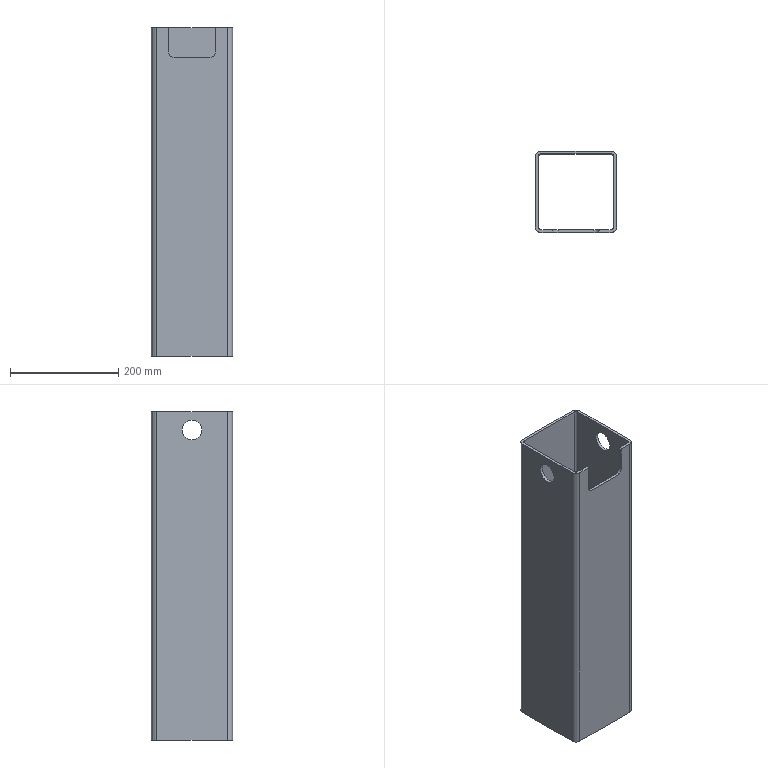Part | SolidWorks | features Fillet 3, ICE 2, Extrusion 1 | 1 solid | 27 faces | box 150 x 150 x 608 mm | volume 1690442 mm3 | cylinder 14 | plane 13 | commonest cylinder face diameters 20 x6 10 x4 36 x4
STEP:
#1=CARTESIAN_POINT('',(5.,75.,592.));
#2=VERTEX_POINT('',#1);
#3=CARTESIAN_POINT('',(5.,75.,556.));
#4=VERTEX_POINT('',#3);
#5=CARTESIAN_POINT('',(5.,75.,574.));
#6=DIRECTION('',(1.,0.,0.));
#7=DIRECTION('',(0.,1.,0.));
#8=AXIS2_PLACEMENT_3D('',#5,#6,#7);
#9=CIRCLE('',#8,18.);
#10=EDGE_CURVE('',#2,#4,#9,.T.);
#11=ORIENTED_EDGE('',*,*,#10,.T.);
#12=CARTESIAN_POINT('',(0.,75.,556.));
#13=VERTEX_POINT('',#12);
#14=CARTESIAN_POINT('',(150.,75.,556.));
#15=DIRECTION('',(-1.,0.,0.));
#16=VECTOR('',#15,1000.);
#17=LINE('',#14,#16);
#18=EDGE_CURVE('',#4,#13,#17,.T.);
#19=ORIENTED_EDGE('',*,*,#18,.T.);
#20=CARTESIAN_POINT('',(0.,75.,592.));
#21=VERTEX_POINT('',#20);
#22=CARTESIAN_POINT('',(0.,75.,574.));
#23=DIRECTION('',(-1.,0.,0.));
#24=DIRECTION('',(0.,0.,1.));
#25=AXIS2_PLACEMENT_3D('',#22,#23,#24);
#26=CIRCLE('',#25,18.);
#27=EDGE_CURVE('',#13,#21,#26,.T.);
#28=ORIENTED_EDGE('',*,*,#27,.T.);
#29=CARTESIAN_POINT('',(150.,75.,592.));
#30=DIRECTION('',(-1.,0.,0.));
#31=VECTOR('',#30,1000.);
#32=LINE('',#29,#31);
#33=EDGE_CURVE('',#2,#21,#32,.T.);
#34=ORIENTED_EDGE('',*,*,#33,.F.);
#35=EDGE_LOOP('',(#11,#19,#28,#34));
#36=FACE_OUTER_BOUND('',#35,.T.);
#37=CARTESIAN_POINT('',(150.,75.,574.));
#38=DIRECTION('',(-1.,0.,0.));
#39=DIRECTION('',(0.,0.,1.));
#40=AXIS2_PLACEMENT_3D('',#37,#38,#39);
#41=CYLINDRICAL_SURFACE('',#40,18.);
#42=ADVANCED_FACE('',(#36),#41,.F.);
#43=CARTESIAN_POINT('',(150.,75.,556.));
#44=VERTEX_POINT('',#43);
#45=CARTESIAN_POINT('',(150.,75.,592.));
#46=VERTEX_POINT('',#45);
#47=CARTESIAN_POINT('',(150.,75.,574.));
#48=DIRECTION('',(-1.,0.,0.));
#49=DIRECTION('',(0.,0.,1.));
#50=AXIS2_PLACEMENT_3D('',#47,#48,#49);
#51=CIRCLE('',#50,18.);
#52=EDGE_CURVE('',#44,#46,#51,.T.);
#53=ORIENTED_EDGE('',*,*,#52,.F.);
#54=CARTESIAN_POINT('',(145.,75.,556.));
#55=VERTEX_POINT('',#54);
#56=CARTESIAN_POINT('',(150.,75.,556.));
#57=DIRECTION('',(-1.,0.,0.));
#58=VECTOR('',#57,1000.);
#59=LINE('',#56,#58);
#60=EDGE_CURVE('',#44,#55,#59,.T.);
#61=ORIENTED_EDGE('',*,*,#60,.T.);
#62=CARTESIAN_POINT('',(145.,75.,592.));
#63=VERTEX_POINT('',#62);
#64=CARTESIAN_POINT('',(145.,75.,574.));
#65=DIRECTION('',(-1.,0.,0.));
#66=DIRECTION('',(0.,-1.,0.));
#67=AXIS2_PLACEMENT_3D('',#64,#65,#66);
#68=CIRCLE('',#67,18.);
#69=EDGE_CURVE('',#55,#63,#68,.T.);
#70=ORIENTED_EDGE('',*,*,#69,.T.);
#71=CARTESIAN_POINT('',(150.,75.,592.));
#72=DIRECTION('',(-1.,0.,0.));
#73=VECTOR('',#72,1000.);
#74=LINE('',#71,#73);
#75=EDGE_CURVE('',#46,#63,#74,.T.);
#76=ORIENTED_EDGE('',*,*,#75,.F.);
#77=EDGE_LOOP('',(#53,#61,#70,#76));
#78=FACE_OUTER_BOUND('',#77,.T.);
#79=CARTESIAN_POINT('',(150.,75.,574.));
#80=DIRECTION('',(-1.,0.,0.));
#81=DIRECTION('',(0.,0.,1.));
#82=AXIS2_PLACEMENT_3D('',#79,#80,#81);
#83=CYLINDRICAL_SURFACE('',#82,18.);
#84=ADVANCED_FACE('',(#78),#83,.F.);
#85=CARTESIAN_POINT('',(10.,0.,608.));
#86=VERTEX_POINT('',#85);
#87=CARTESIAN_POINT('',(32.,0.,608.));
#88=VERTEX_POINT('',#87);
#89=CARTESIAN_POINT('',(0.,0.,608.));
#90=DIRECTION('',(1.,0.,0.));
#91=VECTOR('',#90,1000.);
#92=LINE('',#89,#91);
#93=EDGE_CURVE('',#86,#88,#92,.T.);
#94=ORIENTED_EDGE('',*,*,#93,.T.);
#95=CARTESIAN_POINT('',(32.,5.,608.));
#96=VERTEX_POINT('',#95);
#97=CARTESIAN_POINT('',(32.,10.,608.));
#98=DIRECTION('',(0.,-1.,0.));
#99=VECTOR('',#98,1000.);
#100=LINE('',#97,#99);
#101=EDGE_CURVE('',#96,#88,#100,.T.);
#102=ORIENTED_EDGE('',*,*,#101,.F.);
#103=CARTESIAN_POINT('',(10.,5.,608.));
#104=VERTEX_POINT('',#103);
#105=CARTESIAN_POINT('',(5.,5.,608.));
#106=DIRECTION('',(1.,0.,0.));
#107=VECTOR('',#106,1000.);
#108=LINE('',#105,#107);
#109=EDGE_CURVE('',#104,#96,#108,.T.);
#110=ORIENTED_EDGE('',*,*,#109,.F.);
#111=CARTESIAN_POINT('',(5.,10.,608.));
#112=VERTEX_POINT('',#111);
#113=CARTESIAN_POINT('',(10.,10.,608.));
#114=DIRECTION('',(0.,0.,-1.));
#115=DIRECTION('',(-1.,0.,0.));
#116=AXIS2_PLACEMENT_3D('',#113,#114,#115);
#117=CIRCLE('',#116,5.);
#118=EDGE_CURVE('',#104,#112,#117,.T.);
#119=ORIENTED_EDGE('',*,*,#118,.T.);
#120=CARTESIAN_POINT('',(5.,140.,608.));
#121=VERTEX_POINT('',#120);
#122=CARTESIAN_POINT('',(5.,145.,608.));
#123=DIRECTION('',(0.,-1.,0.));
#124=VECTOR('',#123,1000.);
#125=LINE('',#122,#124);
#126=EDGE_CURVE('',#121,#112,#125,.T.);
#127=ORIENTED_EDGE('',*,*,#126,.F.);
#128=CARTESIAN_POINT('',(10.,145.,608.));
#129=VERTEX_POINT('',#128);
#130=CARTESIAN_POINT('',(10.,140.,608.));
#131=DIRECTION('',(0.,0.,-1.));
#132=DIRECTION('',(-1.,0.,0.));
#133=AXIS2_PLACEMENT_3D('',#130,#131,#132);
#134=CIRCLE('',#133,5.);
#135=EDGE_CURVE('',#121,#129,#134,.T.);
#136=ORIENTED_EDGE('',*,*,#135,.T.);
#137=CARTESIAN_POINT('',(140.,145.,608.));
#138=VERTEX_POINT('',#137);
#139=CARTESIAN_POINT('',(5.,145.,608.));
#140=DIRECTION('',(-1.,0.,0.));
#141=VECTOR('',#140,1000.);
#142=LINE('',#139,#141);
#143=EDGE_CURVE('',#138,#129,#142,.T.);
#144=ORIENTED_EDGE('',*,*,#143,.F.);
#145=CARTESIAN_POINT('',(145.,140.,608.));
#146=VERTEX_POINT('',#145);
#147=CARTESIAN_POINT('',(140.,140.,608.));
#148=DIRECTION('',(0.,0.,-1.));
#149=DIRECTION('',(-1.,0.,0.));
#150=AXIS2_PLACEMENT_3D('',#147,#148,#149);
#151=CIRCLE('',#150,5.);
#152=EDGE_CURVE('',#138,#146,#151,.T.);
#153=ORIENTED_EDGE('',*,*,#152,.T.);
#154=CARTESIAN_POINT('',(145.,10.,608.));
#155=VERTEX_POINT('',#154);
#156=CARTESIAN_POINT('',(145.,145.,608.));
#157=DIRECTION('',(0.,1.,0.));
#158=VECTOR('',#157,1000.);
#159=LINE('',#156,#158);
#160=EDGE_CURVE('',#155,#146,#159,.T.);
#161=ORIENTED_EDGE('',*,*,#160,.F.);
#162=CARTESIAN_POINT('',(140.,5.,608.));
#163=VERTEX_POINT('',#162);
#164=CARTESIAN_POINT('',(140.,10.,608.));
#165=DIRECTION('',(0.,0.,-1.));
#166=DIRECTION('',(-1.,0.,0.));
#167=AXIS2_PLACEMENT_3D('',#164,#165,#166);
#168=CIRCLE('',#167,5.);
#169=EDGE_CURVE('',#155,#163,#168,.T.);
#170=ORIENTED_EDGE('',*,*,#169,.T.);
#171=CARTESIAN_POINT('',(118.,5.,608.));
#172=VERTEX_POINT('',#171);
#173=CARTESIAN_POINT('',(5.,5.,608.));
#174=DIRECTION('',(1.,0.,0.));
#175=VECTOR('',#174,1000.);
#176=LINE('',#173,#175);
#177=EDGE_CURVE('',#172,#163,#176,.T.);
#178=ORIENTED_EDGE('',*,*,#177,.F.);
#179=CARTESIAN_POINT('',(118.,0.,608.));
#180=VERTEX_POINT('',#179);
#181=CARTESIAN_POINT('',(118.,10.,608.));
#182=DIRECTION('',(0.,-1.,0.));
#183=VECTOR('',#182,1000.);
#184=LINE('',#181,#183);
#185=EDGE_CURVE('',#172,#180,#184,.T.);
#186=ORIENTED_EDGE('',*,*,#185,.T.);
#187=CARTESIAN_POINT('',(140.,0.,608.));
#188=VERTEX_POINT('',#187);
#189=CARTESIAN_POINT('',(0.,0.,608.));
#190=DIRECTION('',(1.,0.,0.));
#191=VECTOR('',#190,1000.);
#192=LINE('',#189,#191);
#193=EDGE_CURVE('',#180,#188,#192,.T.);
#194=ORIENTED_EDGE('',*,*,#193,.T.);
#195=CARTESIAN_POINT('',(150.,10.,608.));
#196=VERTEX_POINT('',#195);
#197=CARTESIAN_POINT('',(140.,10.,608.));
#198=DIRECTION('',(0.,0.,1.));
#199=DIRECTION('',(-1.,0.,0.));
#200=AXIS2_PLACEMENT_3D('',#197,#198,#199);
#201=CIRCLE('',#200,10.);
#202=EDGE_CURVE('',#188,#196,#201,.T.);
#203=ORIENTED_EDGE('',*,*,#202,.T.);
#204=CARTESIAN_POINT('',(150.,140.,608.));
#205=VERTEX_POINT('',#204);
#206=CARTESIAN_POINT('',(150.,0.,608.));
#207=DIRECTION('',(0.,1.,0.));
#208=VECTOR('',#207,1000.);
#209=LINE('',#206,#208);
#210=EDGE_CURVE('',#196,#205,#209,.T.);
#211=ORIENTED_EDGE('',*,*,#210,.T.);
#212=CARTESIAN_POINT('',(140.,150.,608.));
#213=VERTEX_POINT('',#212);
#214=CARTESIAN_POINT('',(140.,140.,608.));
#215=DIRECTION('',(0.,0.,1.));
#216=DIRECTION('',(-1.,0.,0.));
#217=AXIS2_PLACEMENT_3D('',#214,#215,#216);
#218=CIRCLE('',#217,10.);
#219=EDGE_CURVE('',#205,#213,#218,.T.);
#220=ORIENTED_EDGE('',*,*,#219,.T.);
#221=CARTESIAN_POINT('',(10.,150.,608.));
#222=VERTEX_POINT('',#221);
#223=CARTESIAN_POINT('',(0.,150.,608.));
#224=DIRECTION('',(-1.,0.,0.));
#225=VECTOR('',#224,1000.);
#226=LINE('',#223,#225);
#227=EDGE_CURVE('',#213,#222,#226,.T.);
#228=ORIENTED_EDGE('',*,*,#227,.T.);
#229=CARTESIAN_POINT('',(0.,140.,608.));
#230=VERTEX_POINT('',#229);
#231=CARTESIAN_POINT('',(10.,140.,608.));
#232=DIRECTION('',(0.,0.,1.));
#233=DIRECTION('',(-1.,0.,0.));
#234=AXIS2_PLACEMENT_3D('',#231,#232,#233);
#235=CIRCLE('',#234,10.);
#236=EDGE_CURVE('',#222,#230,#235,.T.);
#237=ORIENTED_EDGE('',*,*,#236,.T.);
#238=CARTESIAN_POINT('',(0.,10.,608.));
#239=VERTEX_POINT('',#238);
#240=CARTESIAN_POINT('',(0.,0.,608.));
#241=DIRECTION('',(0.,-1.,0.));
#242=VECTOR('',#241,1000.);
#243=LINE('',#240,#242);
#244=EDGE_CURVE('',#230,#239,#243,.T.);
#245=ORIENTED_EDGE('',*,*,#244,.T.);
#246=CARTESIAN_POINT('',(10.,10.,608.));
#247=DIRECTION('',(0.,0.,1.));
#248=DIRECTION('',(-1.,0.,0.));
#249=AXIS2_PLACEMENT_3D('',#246,#247,#248);
#250=CIRCLE('',#249,10.);
#251=EDGE_CURVE('',#239,#86,#250,.T.);
#252=ORIENTED_EDGE('',*,*,#251,.T.);
#253=EDGE_LOOP('',(#94,#102,#110,#119,#127,#136,#144,#153,#161,#170,#178,#186,#194,#203,#211,#220,#228,#237,#245,#252));
#254=FACE_OUTER_BOUND('',#253,.T.);
#255=CARTESIAN_POINT('',(0.,0.,608.));
#256=DIRECTION('',(0.,0.,-1.));
#257=DIRECTION('',(-1.,0.,0.));
#258=AXIS2_PLACEMENT_3D('',#255,#256,#257);
#259=PLANE('',#258);
#260=ADVANCED_FACE('',(#254),#259,.F.);
#261=CARTESIAN_POINT('',(150.,10.,0.));
#262=VERTEX_POINT('',#261);
#263=CARTESIAN_POINT('',(150.,140.,0.));
#264=VERTEX_POINT('',#263);
#265=CARTESIAN_POINT('',(150.,0.,0.));
#266=DIRECTION('',(0.,1.,0.));
#267=VECTOR('',#266,1000.);
#268=LINE('',#265,#267);
#269=EDGE_CURVE('',#262,#264,#268,.T.);
#270=ORIENTED_EDGE('',*,*,#269,.F.);
#271=CARTESIAN_POINT('',(140.,0.,0.));
#272=VERTEX_POINT('',#271);
#273=CARTESIAN_POINT('',(140.,10.,0.));
#274=DIRECTION('',(0.,0.,-1.));
#275=DIRECTION('',(-1.,0.,0.));
#276=AXIS2_PLACEMENT_3D('',#273,#274,#275);
#277=CIRCLE('',#276,10.);
#278=EDGE_CURVE('',#262,#272,#277,.T.);
#279=ORIENTED_EDGE('',*,*,#278,.T.);
#280=CARTESIAN_POINT('',(10.,0.,0.));
#281=VERTEX_POINT('',#280);
#282=CARTESIAN_POINT('',(0.,0.,0.));
#283=DIRECTION('',(1.,0.,0.));
#284=VECTOR('',#283,1000.);
#285=LINE('',#282,#284);
#286=EDGE_CURVE('',#281,#272,#285,.T.);
#287=ORIENTED_EDGE('',*,*,#286,.F.);
#288=CARTESIAN_POINT('',(0.,10.,0.));
#289=VERTEX_POINT('',#288);
#290=CARTESIAN_POINT('',(10.,10.,0.));
#291=DIRECTION('',(0.,0.,-1.));
#292=DIRECTION('',(-1.,0.,0.));
#293=AXIS2_PLACEMENT_3D('',#290,#291,#292);
#294=CIRCLE('',#293,10.);
#295=EDGE_CURVE('',#281,#289,#294,.T.);
#296=ORIENTED_EDGE('',*,*,#295,.T.);
#297=CARTESIAN_POINT('',(0.,140.,0.));
#298=VERTEX_POINT('',#297);
#299=CARTESIAN_POINT('',(0.,0.,0.));
#300=DIRECTION('',(0.,-1.,0.));
#301=VECTOR('',#300,1000.);
#302=LINE('',#299,#301);
#303=EDGE_CURVE('',#298,#289,#302,.T.);
#304=ORIENTED_EDGE('',*,*,#303,.F.);
#305=CARTESIAN_POINT('',(10.,150.,0.));
#306=VERTEX_POINT('',#305);
#307=CARTESIAN_POINT('',(10.,140.,0.));
#308=DIRECTION('',(0.,0.,-1.));
#309=DIRECTION('',(-1.,0.,0.));
#310=AXIS2_PLACEMENT_3D('',#307,#308,#309);
#311=CIRCLE('',#310,10.);
#312=EDGE_CURVE('',#298,#306,#311,.T.);
#313=ORIENTED_EDGE('',*,*,#312,.T.);
#314=CARTESIAN_POINT('',(140.,150.,0.));
#315=VERTEX_POINT('',#314);
#316=CARTESIAN_POINT('',(0.,150.,0.));
#317=DIRECTION('',(-1.,0.,0.));
#318=VECTOR('',#317,1000.);
#319=LINE('',#316,#318);
#320=EDGE_CURVE('',#315,#306,#319,.T.);
#321=ORIENTED_EDGE('',*,*,#320,.F.);
#322=CARTESIAN_POINT('',(140.,140.,0.));
#323=DIRECTION('',(0.,0.,-1.));
#324=DIRECTION('',(-1.,0.,0.));
#325=AXIS2_PLACEMENT_3D('',#322,#323,#324);
#326=CIRCLE('',#325,10.);
#327=EDGE_CURVE('',#315,#264,#326,.T.);
#328=ORIENTED_EDGE('',*,*,#327,.T.);
#329=EDGE_LOOP('',(#270,#279,#287,#296,#304,#313,#321,#328));
#330=FACE_OUTER_BOUND('',#329,.T.);
#331=CARTESIAN_POINT('',(145.,10.,0.));
#332=VERTEX_POINT('',#331);
#333=CARTESIAN_POINT('',(145.,140.,0.));
#334=VERTEX_POINT('',#333);
#335=CARTESIAN_POINT('',(145.,145.,0.));
#336=DIRECTION('',(0.,1.,0.));
#337=VECTOR('',#336,1000.);
#338=LINE('',#335,#337);
#339=EDGE_CURVE('',#332,#334,#338,.T.);
#340=ORIENTED_EDGE('',*,*,#339,.T.);
#341=CARTESIAN_POINT('',(140.,145.,0.));
#342=VERTEX_POINT('',#341);
#343=CARTESIAN_POINT('',(140.,140.,0.));
#344=DIRECTION('',(0.,0.,1.));
#345=DIRECTION('',(-1.,0.,0.));
#346=AXIS2_PLACEMENT_3D('',#343,#344,#345);
#347=CIRCLE('',#346,5.);
#348=EDGE_CURVE('',#334,#342,#347,.T.);
#349=ORIENTED_EDGE('',*,*,#348,.T.);
#350=CARTESIAN_POINT('',(10.,145.,0.));
#351=VERTEX_POINT('',#350);
#352=CARTESIAN_POINT('',(5.,145.,0.));
#353=DIRECTION('',(-1.,0.,0.));
#354=VECTOR('',#353,1000.);
#355=LINE('',#352,#354);
#356=EDGE_CURVE('',#342,#351,#355,.T.);
#357=ORIENTED_EDGE('',*,*,#356,.T.);
#358=CARTESIAN_POINT('',(5.,140.,0.));
#359=VERTEX_POINT('',#358);
#360=CARTESIAN_POINT('',(10.,140.,0.));
#361=DIRECTION('',(0.,0.,1.));
#362=DIRECTION('',(-1.,0.,0.));
#363=AXIS2_PLACEMENT_3D('',#360,#361,#362);
#364=CIRCLE('',#363,5.);
#365=EDGE_CURVE('',#351,#359,#364,.T.);
#366=ORIENTED_EDGE('',*,*,#365,.T.);
#367=CARTESIAN_POINT('',(5.,10.,0.));
#368=VERTEX_POINT('',#367);
#369=CARTESIAN_POINT('',(5.,145.,0.));
#370=DIRECTION('',(0.,-1.,0.));
#371=VECTOR('',#370,1000.);
#372=LINE('',#369,#371);
#373=EDGE_CURVE('',#359,#368,#372,.T.);
#374=ORIENTED_EDGE('',*,*,#373,.T.);
#375=CARTESIAN_POINT('',(10.,5.,0.));
#376=VERTEX_POINT('',#375);
#377=CARTESIAN_POINT('',(10.,10.,0.));
#378=DIRECTION('',(0.,0.,1.));
#379=DIRECTION('',(-1.,0.,0.));
#380=AXIS2_PLACEMENT_3D('',#377,#378,#379);
#381=CIRCLE('',#380,5.);
#382=EDGE_CURVE('',#368,#376,#381,.T.);
#383=ORIENTED_EDGE('',*,*,#382,.T.);
#384=CARTESIAN_POINT('',(140.,5.,0.));
#385=VERTEX_POINT('',#384);
#386=CARTESIAN_POINT('',(5.,5.,0.));
#387=DIRECTION('',(1.,0.,0.));
#388=VECTOR('',#387,1000.);
#389=LINE('',#386,#388);
#390=EDGE_CURVE('',#376,#385,#389,.T.);
#391=ORIENTED_EDGE('',*,*,#390,.T.);
#392=CARTESIAN_POINT('',(140.,10.,0.));
#393=DIRECTION('',(0.,0.,1.));
#394=DIRECTION('',(-1.,0.,0.));
#395=AXIS2_PLACEMENT_3D('',#392,#393,#394);
#396=CIRCLE('',#395,5.);
#397=EDGE_CURVE('',#385,#332,#396,.T.);
#398=ORIENTED_EDGE('',*,*,#397,.T.);
#399=EDGE_LOOP('',(#340,#349,#357,#366,#374,#383,#391,#398));
#400=FACE_BOUND('',#399,.T.);
#401=CARTESIAN_POINT('',(0.,0.,0.));
#402=DIRECTION('',(0.,0.,-1.));
#403=DIRECTION('',(-1.,0.,0.));
#404=AXIS2_PLACEMENT_3D('',#401,#402,#403);
#405=PLANE('',#404);
#406=ADVANCED_FACE('',(#330,#400),#405,.T.);
#407=CARTESIAN_POINT('',(0.,75.,574.));
#408=DIRECTION('',(-1.,0.,0.));
#409=DIRECTION('',(0.,0.,1.));
#410=AXIS2_PLACEMENT_3D('',#407,#408,#409);
#411=CIRCLE('',#410,18.);
#412=EDGE_CURVE('',#21,#13,#411,.T.);
#413=ORIENTED_EDGE('',*,*,#412,.F.);
#414=ORIENTED_EDGE('',*,*,#27,.F.);
#415=EDGE_LOOP('',(#413,#414));
#416=FACE_BOUND('',#415,.T.);
#417=ORIENTED_EDGE('',*,*,#303,.T.);
#418=CARTESIAN_POINT('',(0.,10.,608.));
#419=DIRECTION('',(0.,0.,1.));
#420=VECTOR('',#419,1000.);
#421=LINE('',#418,#420);
#422=EDGE_CURVE('',#289,#239,#421,.T.);
#423=ORIENTED_EDGE('',*,*,#422,.T.);
#424=ORIENTED_EDGE('',*,*,#244,.F.);
#425=CARTESIAN_POINT('',(0.,140.,608.));
#426=DIRECTION('',(0.,0.,-1.));
#427=VECTOR('',#426,1000.);
#428=LINE('',#425,#427);
#429=EDGE_CURVE('',#230,#298,#428,.T.);
#430=ORIENTED_EDGE('',*,*,#429,.T.);
#431=EDGE_LOOP('',(#417,#423,#424,#430));
#432=FACE_OUTER_BOUND('',#431,.T.);
#433=CARTESIAN_POINT('',(0.,0.,608.));
#434=DIRECTION('',(1.,0.,0.));
#435=DIRECTION('',(0.,0.,-1.));
#436=AXIS2_PLACEMENT_3D('',#433,#434,#435);
#437=PLANE('',#436);
#438=ADVANCED_FACE('',(#416,#432),#437,.F.);
#439=CARTESIAN_POINT('',(42.,0.,553.));
#440=VERTEX_POINT('',#439);
#441=CARTESIAN_POINT('',(108.,0.,553.));
#442=VERTEX_POINT('',#441);
#443=CARTESIAN_POINT('',(32.,0.,553.));
#444=DIRECTION('',(1.,0.,0.));
#445=VECTOR('',#444,1000.);
#446=LINE('',#443,#445);
#447=EDGE_CURVE('',#440,#442,#446,.T.);
#448=ORIENTED_EDGE('',*,*,#447,.F.);
#449=CARTESIAN_POINT('',(32.,0.,563.));
#450=VERTEX_POINT('',#449);
#451=CARTESIAN_POINT('',(42.,0.,563.));
#452=DIRECTION('',(0.,1.,0.));
#453=DIRECTION('',(0.,0.,1.));
#454=AXIS2_PLACEMENT_3D('',#451,#452,#453);
#455=CIRCLE('',#454,10.);
#456=EDGE_CURVE('',#440,#450,#455,.T.);
#457=ORIENTED_EDGE('',*,*,#456,.T.);
#458=CARTESIAN_POINT('',(32.,0.,608.));
#459=DIRECTION('',(0.,0.,-1.));
#460=VECTOR('',#459,1000.);
#461=LINE('',#458,#460);
#462=EDGE_CURVE('',#88,#450,#461,.T.);
#463=ORIENTED_EDGE('',*,*,#462,.F.);
#464=ORIENTED_EDGE('',*,*,#93,.F.);
#465=CARTESIAN_POINT('',(10.,0.,608.));
#466=DIRECTION('',(0.,0.,-1.));
#467=VECTOR('',#466,1000.);
#468=LINE('',#465,#467);
#469=EDGE_CURVE('',#86,#281,#468,.T.);
#470=ORIENTED_EDGE('',*,*,#469,.T.);
#471=ORIENTED_EDGE('',*,*,#286,.T.);
#472=CARTESIAN_POINT('',(140.,0.,608.));
#473=DIRECTION('',(0.,0.,1.));
#474=VECTOR('',#473,1000.);
#475=LINE('',#472,#474);
#476=EDGE_CURVE('',#272,#188,#475,.T.);
#477=ORIENTED_EDGE('',*,*,#476,.T.);
#478=ORIENTED_EDGE('',*,*,#193,.F.);
#479=CARTESIAN_POINT('',(118.,0.,563.));
#480=VERTEX_POINT('',#479);
#481=CARTESIAN_POINT('',(118.,0.,608.));
#482=DIRECTION('',(0.,0.,1.));
#483=VECTOR('',#482,1000.);
#484=LINE('',#481,#483);
#485=EDGE_CURVE('',#480,#180,#484,.T.);
#486=ORIENTED_EDGE('',*,*,#485,.F.);
#487=CARTESIAN_POINT('',(108.,0.,563.));
#488=DIRECTION('',(0.,1.,0.));
#489=DIRECTION('',(0.,0.,1.));
#490=AXIS2_PLACEMENT_3D('',#487,#488,#489);
#491=CIRCLE('',#490,10.);
#492=EDGE_CURVE('',#480,#442,#491,.T.);
#493=ORIENTED_EDGE('',*,*,#492,.T.);
#494=EDGE_LOOP('',(#448,#457,#463,#464,#470,#471,#477,#478,#486,#493));
#495=FACE_OUTER_BOUND('',#494,.T.);
#496=CARTESIAN_POINT('',(0.,0.,608.));
#497=DIRECTION('',(0.,1.,0.));
#498=DIRECTION('',(0.,0.,1.));
#499=AXIS2_PLACEMENT_3D('',#496,#497,#498);
#500=PLANE('',#499);
#501=ADVANCED_FACE('',(#495),#500,.F.);
#502=CARTESIAN_POINT('',(150.,75.,574.));
#503=DIRECTION('',(-1.,0.,0.));
#504=DIRECTION('',(0.,0.,1.));
#505=AXIS2_PLACEMENT_3D('',#502,#503,#504);
#506=CIRCLE('',#505,18.);
#507=EDGE_CURVE('',#46,#44,#506,.T.);
#508=ORIENTED_EDGE('',*,*,#507,.T.);
#509=ORIENTED_EDGE('',*,*,#52,.T.);
#510=EDGE_LOOP('',(#508,#509));
#511=FACE_BOUND('',#510,.T.);
#512=ORIENTED_EDGE('',*,*,#210,.F.);
#513=CARTESIAN_POINT('',(150.,10.,608.));
#514=DIRECTION('',(0.,0.,-1.));
#515=VECTOR('',#514,1000.);
#516=LINE('',#513,#515);
#517=EDGE_CURVE('',#196,#262,#516,.T.);
#518=ORIENTED_EDGE('',*,*,#517,.T.);
#519=ORIENTED_EDGE('',*,*,#269,.T.);
#520=CARTESIAN_POINT('',(150.,140.,608.));
#521=DIRECTION('',(0.,0.,1.));
#522=VECTOR('',#521,1000.);
#523=LINE('',#520,#522);
#524=EDGE_CURVE('',#264,#205,#523,.T.);
#525=ORIENTED_EDGE('',*,*,#524,.T.);
#526=EDGE_LOOP('',(#512,#518,#519,#525));
#527=FACE_OUTER_BOUND('',#526,.T.);
#528=CARTESIAN_POINT('',(150.,0.,608.));
#529=DIRECTION('',(-1.,0.,0.));
#530=DIRECTION('',(0.,0.,1.));
#531=AXIS2_PLACEMENT_3D('',#528,#529,#530);
#532=PLANE('',#531);
#533=ADVANCED_FACE('',(#511,#527),#532,.F.);
#534=ORIENTED_EDGE('',*,*,#320,.T.);
#535=CARTESIAN_POINT('',(10.,150.,608.));
#536=DIRECTION('',(0.,0.,1.));
#537=VECTOR('',#536,1000.);
#538=LINE('',#535,#537);
#539=EDGE_CURVE('',#306,#222,#538,.T.);
#540=ORIENTED_EDGE('',*,*,#539,.T.);
#541=ORIENTED_EDGE('',*,*,#227,.F.);
#542=CARTESIAN_POINT('',(140.,150.,608.));
#543=DIRECTION('',(0.,0.,-1.));
#544=VECTOR('',#543,1000.);
#545=LINE('',#542,#544);
#546=EDGE_CURVE('',#213,#315,#545,.T.);
#547=ORIENTED_EDGE('',*,*,#546,.T.);
#548=EDGE_LOOP('',(#534,#540,#541,#547));
#549=FACE_OUTER_BOUND('',#548,.T.);
#550=CARTESIAN_POINT('',(0.,150.,608.));
#551=DIRECTION('',(0.,-1.,0.));
#552=DIRECTION('',(0.,0.,-1.));
#553=AXIS2_PLACEMENT_3D('',#550,#551,#552);
#554=PLANE('',#553);
#555=ADVANCED_FACE('',(#549),#554,.F.);
#556=ORIENTED_EDGE('',*,*,#10,.F.);
#557=CARTESIAN_POINT('',(5.,75.,574.));
#558=DIRECTION('',(1.,0.,0.));
#559=DIRECTION('',(0.,1.,0.));
#560=AXIS2_PLACEMENT_3D('',#557,#558,#559);
#561=CIRCLE('',#560,18.);
#562=EDGE_CURVE('',#4,#2,#561,.T.);
#563=ORIENTED_EDGE('',*,*,#562,.F.);
#564=EDGE_LOOP('',(#556,#563));
#565=FACE_BOUND('',#564,.T.);
#566=ORIENTED_EDGE('',*,*,#126,.T.);
#567=CARTESIAN_POINT('',(5.,10.,0.));
#568=DIRECTION('',(0.,0.,-1.));
#569=VECTOR('',#568,1000.);
#570=LINE('',#567,#569);
#571=EDGE_CURVE('',#112,#368,#570,.T.);
#572=ORIENTED_EDGE('',*,*,#571,.T.);
#573=ORIENTED_EDGE('',*,*,#373,.F.);
#574=CARTESIAN_POINT('',(5.,140.,608.));
#575=DIRECTION('',(0.,0.,1.));
#576=VECTOR('',#575,1000.);
#577=LINE('',#574,#576);
#578=EDGE_CURVE('',#359,#121,#577,.T.);
#579=ORIENTED_EDGE('',*,*,#578,.T.);
#580=EDGE_LOOP('',(#566,#572,#573,#579));
#581=FACE_OUTER_BOUND('',#580,.T.);
#582=CARTESIAN_POINT('',(5.,145.,608.));
#583=DIRECTION('',(1.,0.,0.));
#584=DIRECTION('',(0.,1.,0.));
#585=AXIS2_PLACEMENT_3D('',#582,#583,#584);
#586=PLANE('',#585);
#587=ADVANCED_FACE('',(#565,#581),#586,.T.);
#588=CARTESIAN_POINT('',(32.,5.,563.));
#589=VERTEX_POINT('',#588);
#590=CARTESIAN_POINT('',(32.,5.,608.));
#591=DIRECTION('',(0.,0.,1.));
#592=VECTOR('',#591,1000.);
#593=LINE('',#590,#592);
#594=EDGE_CURVE('',#589,#96,#593,.T.);
#595=ORIENTED_EDGE('',*,*,#594,.F.);
#596=CARTESIAN_POINT('',(42.,5.,553.));
#597=VERTEX_POINT('',#596);
#598=CARTESIAN_POINT('',(42.,5.,563.));
#599=DIRECTION('',(0.,-1.,0.));
#600=DIRECTION('',(-1.,0.,0.));
#601=AXIS2_PLACEMENT_3D('',#598,#599,#600);
#602=CIRCLE('',#601,10.);
#603=EDGE_CURVE('',#589,#597,#602,.T.);
#604=ORIENTED_EDGE('',*,*,#603,.T.);
#605=CARTESIAN_POINT('',(108.,5.,553.));
#606=VERTEX_POINT('',#605);
#607=CARTESIAN_POINT('',(5.,5.,553.));
#608=DIRECTION('',(-1.,0.,0.));
#609=VECTOR('',#608,1000.);
#610=LINE('',#607,#609);
#611=EDGE_CURVE('',#606,#597,#610,.T.);
#612=ORIENTED_EDGE('',*,*,#611,.F.);
#613=CARTESIAN_POINT('',(118.,5.,563.));
#614=VERTEX_POINT('',#613);
#615=CARTESIAN_POINT('',(108.,5.,563.));
#616=DIRECTION('',(0.,-1.,0.));
#617=DIRECTION('',(-1.,0.,0.));
#618=AXIS2_PLACEMENT_3D('',#615,#616,#617);
#619=CIRCLE('',#618,10.);
#620=EDGE_CURVE('',#606,#614,#619,.T.);
#621=ORIENTED_EDGE('',*,*,#620,.T.);
#622=CARTESIAN_POINT('',(118.,5.,608.));
#623=DIRECTION('',(0.,0.,-1.));
#624=VECTOR('',#623,1000.);
#625=LINE('',#622,#624);
#626=EDGE_CURVE('',#172,#614,#625,.T.);
#627=ORIENTED_EDGE('',*,*,#626,.F.);
#628=ORIENTED_EDGE('',*,*,#177,.T.);
#629=CARTESIAN_POINT('',(140.,5.,0.));
#630=DIRECTION('',(0.,0.,-1.));
#631=VECTOR('',#630,1000.);
#632=LINE('',#629,#631);
#633=EDGE_CURVE('',#163,#385,#632,.T.);
#634=ORIENTED_EDGE('',*,*,#633,.T.);
#635=ORIENTED_EDGE('',*,*,#390,.F.);
#636=CARTESIAN_POINT('',(10.,5.,608.));
#637=DIRECTION('',(0.,0.,1.));
#638=VECTOR('',#637,1000.);
#639=LINE('',#636,#638);
#640=EDGE_CURVE('',#376,#104,#639,.T.);
#641=ORIENTED_EDGE('',*,*,#640,.T.);
#642=ORIENTED_EDGE('',*,*,#109,.T.);
#643=EDGE_LOOP('',(#595,#604,#612,#621,#627,#628,#634,#635,#641,#642));
#644=FACE_OUTER_BOUND('',#643,.T.);
#645=CARTESIAN_POINT('',(5.,5.,608.));
#646=DIRECTION('',(0.,1.,0.));
#647=DIRECTION('',(-1.,0.,0.));
#648=AXIS2_PLACEMENT_3D('',#645,#646,#647);
#649=PLANE('',#648);
#650=ADVANCED_FACE('',(#644),#649,.T.);
#651=CARTESIAN_POINT('',(145.,75.,574.));
#652=DIRECTION('',(-1.,0.,0.));
#653=DIRECTION('',(0.,-1.,0.));
#654=AXIS2_PLACEMENT_3D('',#651,#652,#653);
#655=CIRCLE('',#654,18.);
#656=EDGE_CURVE('',#63,#55,#655,.T.);
#657=ORIENTED_EDGE('',*,*,#656,.F.);
#658=ORIENTED_EDGE('',*,*,#69,.F.);
#659=EDGE_LOOP('',(#657,#658));
#660=FACE_BOUND('',#659,.T.);
#661=ORIENTED_EDGE('',*,*,#339,.F.);
#662=CARTESIAN_POINT('',(145.,10.,608.));
#663=DIRECTION('',(0.,0.,1.));
#664=VECTOR('',#663,1000.);
#665=LINE('',#662,#664);
#666=EDGE_CURVE('',#332,#155,#665,.T.);
#667=ORIENTED_EDGE('',*,*,#666,.T.);
#668=ORIENTED_EDGE('',*,*,#160,.T.);
#669=CARTESIAN_POINT('',(145.,140.,0.));
#670=DIRECTION('',(0.,0.,-1.));
#671=VECTOR('',#670,1000.);
#672=LINE('',#669,#671);
#673=EDGE_CURVE('',#146,#334,#672,.T.);
#674=ORIENTED_EDGE('',*,*,#673,.T.);
#675=EDGE_LOOP('',(#661,#667,#668,#674));
#676=FACE_OUTER_BOUND('',#675,.T.);
#677=CARTESIAN_POINT('',(145.,145.,608.));
#678=DIRECTION('',(-1.,0.,0.));
#679=DIRECTION('',(0.,-1.,0.));
#680=AXIS2_PLACEMENT_3D('',#677,#678,#679);
#681=PLANE('',#680);
#682=ADVANCED_FACE('',(#660,#676),#681,.T.);
#683=ORIENTED_EDGE('',*,*,#356,.F.);
#684=CARTESIAN_POINT('',(140.,145.,608.));
#685=DIRECTION('',(0.,0.,1.));
#686=VECTOR('',#685,1000.);
#687=LINE('',#684,#686);
#688=EDGE_CURVE('',#342,#138,#687,.T.);
#689=ORIENTED_EDGE('',*,*,#688,.T.);
#690=ORIENTED_EDGE('',*,*,#143,.T.);
#691=CARTESIAN_POINT('',(10.,145.,0.));
#692=DIRECTION('',(0.,0.,-1.));
#693=VECTOR('',#692,1000.);
#694=LINE('',#691,#693);
#695=EDGE_CURVE('',#129,#351,#694,.T.);
#696=ORIENTED_EDGE('',*,*,#695,.T.);
#697=EDGE_LOOP('',(#683,#689,#690,#696));
#698=FACE_OUTER_BOUND('',#697,.T.);
#699=CARTESIAN_POINT('',(5.,145.,608.));
#700=DIRECTION('',(0.,-1.,0.));
#701=DIRECTION('',(0.,0.,-1.));
#702=AXIS2_PLACEMENT_3D('',#699,#700,#701);
#703=PLANE('',#702);
#704=ADVANCED_FACE('',(#698),#703,.T.);
#705=ORIENTED_EDGE('',*,*,#202,.F.);
#706=ORIENTED_EDGE('',*,*,#476,.F.);
#707=ORIENTED_EDGE('',*,*,#278,.F.);
#708=ORIENTED_EDGE('',*,*,#517,.F.);
#709=EDGE_LOOP('',(#705,#706,#707,#708));
#710=FACE_OUTER_BOUND('',#709,.T.);
#711=CARTESIAN_POINT('',(140.,10.,608.));
#712=DIRECTION('',(0.,0.,-1.));
#713=DIRECTION('',(-1.,0.,0.));
#714=AXIS2_PLACEMENT_3D('',#711,#712,#713);
#715=CYLINDRICAL_SURFACE('',#714,10.);
#716=ADVANCED_FACE('',(#710),#715,.T.);
#717=ORIENTED_EDGE('',*,*,#251,.F.);
#718=ORIENTED_EDGE('',*,*,#422,.F.);
#719=ORIENTED_EDGE('',*,*,#295,.F.);
#720=ORIENTED_EDGE('',*,*,#469,.F.);
#721=EDGE_LOOP('',(#717,#718,#719,#720));
#722=FACE_OUTER_BOUND('',#721,.T.);
#723=CARTESIAN_POINT('',(10.,10.,608.));
#724=DIRECTION('',(0.,0.,-1.));
#725=DIRECTION('',(-1.,0.,0.));
#726=AXIS2_PLACEMENT_3D('',#723,#724,#725);
#727=CYLINDRICAL_SURFACE('',#726,10.);
#728=ADVANCED_FACE('',(#722),#727,.T.);
#729=ORIENTED_EDGE('',*,*,#236,.F.);
#730=ORIENTED_EDGE('',*,*,#539,.F.);
#731=ORIENTED_EDGE('',*,*,#312,.F.);
#732=ORIENTED_EDGE('',*,*,#429,.F.);
#733=EDGE_LOOP('',(#729,#730,#731,#732));
#734=FACE_OUTER_BOUND('',#733,.T.);
#735=CARTESIAN_POINT('',(10.,140.,608.));
#736=DIRECTION('',(0.,0.,-1.));
#737=DIRECTION('',(-1.,0.,0.));
#738=AXIS2_PLACEMENT_3D('',#735,#736,#737);
#739=CYLINDRICAL_SURFACE('',#738,10.);
#740=ADVANCED_FACE('',(#734),#739,.T.);
#741=ORIENTED_EDGE('',*,*,#219,.F.);
#742=ORIENTED_EDGE('',*,*,#524,.F.);
#743=ORIENTED_EDGE('',*,*,#327,.F.);
#744=ORIENTED_EDGE('',*,*,#546,.F.);
#745=EDGE_LOOP('',(#741,#742,#743,#744));
#746=FACE_OUTER_BOUND('',#745,.T.);
#747=CARTESIAN_POINT('',(140.,140.,608.));
#748=DIRECTION('',(0.,0.,-1.));
#749=DIRECTION('',(-1.,0.,0.));
#750=AXIS2_PLACEMENT_3D('',#747,#748,#749);
#751=CYLINDRICAL_SURFACE('',#750,10.);
#752=ADVANCED_FACE('',(#746),#751,.T.);
#753=ORIENTED_EDGE('',*,*,#118,.F.);
#754=ORIENTED_EDGE('',*,*,#640,.F.);
#755=ORIENTED_EDGE('',*,*,#382,.F.);
#756=ORIENTED_EDGE('',*,*,#571,.F.);
#757=EDGE_LOOP('',(#753,#754,#755,#756));
#758=FACE_OUTER_BOUND('',#757,.T.);
#759=CARTESIAN_POINT('',(10.,10.,608.));
#760=DIRECTION('',(0.,0.,1.));
#761=DIRECTION('',(1.,0.,0.));
#762=AXIS2_PLACEMENT_3D('',#759,#760,#761);
#763=CYLINDRICAL_SURFACE('',#762,5.);
#764=ADVANCED_FACE('',(#758),#763,.F.);
#765=ORIENTED_EDGE('',*,*,#169,.F.);
#766=ORIENTED_EDGE('',*,*,#666,.F.);
#767=ORIENTED_EDGE('',*,*,#397,.F.);
#768=ORIENTED_EDGE('',*,*,#633,.F.);
#769=EDGE_LOOP('',(#765,#766,#767,#768));
#770=FACE_OUTER_BOUND('',#769,.T.);
#771=CARTESIAN_POINT('',(140.,10.,608.));
#772=DIRECTION('',(0.,0.,1.));
#773=DIRECTION('',(1.,0.,0.));
#774=AXIS2_PLACEMENT_3D('',#771,#772,#773);
#775=CYLINDRICAL_SURFACE('',#774,5.);
#776=ADVANCED_FACE('',(#770),#775,.F.);
#777=ORIENTED_EDGE('',*,*,#152,.F.);
#778=ORIENTED_EDGE('',*,*,#688,.F.);
#779=ORIENTED_EDGE('',*,*,#348,.F.);
#780=ORIENTED_EDGE('',*,*,#673,.F.);
#781=EDGE_LOOP('',(#777,#778,#779,#780));
#782=FACE_OUTER_BOUND('',#781,.T.);
#783=CARTESIAN_POINT('',(140.,140.,608.));
#784=DIRECTION('',(0.,0.,1.));
#785=DIRECTION('',(1.,0.,0.));
#786=AXIS2_PLACEMENT_3D('',#783,#784,#785);
#787=CYLINDRICAL_SURFACE('',#786,5.);
#788=ADVANCED_FACE('',(#782),#787,.F.);
#789=ORIENTED_EDGE('',*,*,#135,.F.);
#790=ORIENTED_EDGE('',*,*,#578,.F.);
#791=ORIENTED_EDGE('',*,*,#365,.F.);
#792=ORIENTED_EDGE('',*,*,#695,.F.);
#793=EDGE_LOOP('',(#789,#790,#791,#792));
#794=FACE_OUTER_BOUND('',#793,.T.);
#795=CARTESIAN_POINT('',(10.,140.,608.));
#796=DIRECTION('',(0.,0.,1.));
#797=DIRECTION('',(1.,0.,0.));
#798=AXIS2_PLACEMENT_3D('',#795,#796,#797);
#799=CYLINDRICAL_SURFACE('',#798,5.);
#800=ADVANCED_FACE('',(#794),#799,.F.);
#801=ORIENTED_EDGE('',*,*,#60,.F.);
#802=ORIENTED_EDGE('',*,*,#507,.F.);
#803=ORIENTED_EDGE('',*,*,#75,.T.);
#804=ORIENTED_EDGE('',*,*,#656,.T.);
#805=EDGE_LOOP('',(#801,#802,#803,#804));
#806=FACE_OUTER_BOUND('',#805,.T.);
#807=CARTESIAN_POINT('',(150.,75.,574.));
#808=DIRECTION('',(-1.,0.,0.));
#809=DIRECTION('',(0.,0.,1.));
#810=AXIS2_PLACEMENT_3D('',#807,#808,#809);
#811=CYLINDRICAL_SURFACE('',#810,18.);
#812=ADVANCED_FACE('',(#806),#811,.F.);
#813=ORIENTED_EDGE('',*,*,#18,.F.);
#814=ORIENTED_EDGE('',*,*,#562,.T.);
#815=ORIENTED_EDGE('',*,*,#33,.T.);
#816=ORIENTED_EDGE('',*,*,#412,.T.);
#817=EDGE_LOOP('',(#813,#814,#815,#816));
#818=FACE_OUTER_BOUND('',#817,.T.);
#819=CARTESIAN_POINT('',(150.,75.,574.));
#820=DIRECTION('',(-1.,0.,0.));
#821=DIRECTION('',(0.,0.,1.));
#822=AXIS2_PLACEMENT_3D('',#819,#820,#821);
#823=CYLINDRICAL_SURFACE('',#822,18.);
#824=ADVANCED_FACE('',(#818),#823,.F.);
#825=ORIENTED_EDGE('',*,*,#462,.T.);
#826=CARTESIAN_POINT('',(32.,5.,563.));
#827=DIRECTION('',(0.,1.,0.));
#828=VECTOR('',#827,1000.);
#829=LINE('',#826,#828);
#830=EDGE_CURVE('',#450,#589,#829,.T.);
#831=ORIENTED_EDGE('',*,*,#830,.T.);
#832=ORIENTED_EDGE('',*,*,#594,.T.);
#833=ORIENTED_EDGE('',*,*,#101,.T.);
#834=EDGE_LOOP('',(#825,#831,#832,#833));
#835=FACE_OUTER_BOUND('',#834,.T.);
#836=CARTESIAN_POINT('',(32.,10.,608.));
#837=DIRECTION('',(-1.,0.,0.));
#838=DIRECTION('',(0.,0.,1.));
#839=AXIS2_PLACEMENT_3D('',#836,#837,#838);
#840=PLANE('',#839);
#841=ADVANCED_FACE('',(#835),#840,.F.);
#842=ORIENTED_EDGE('',*,*,#626,.T.);
#843=CARTESIAN_POINT('',(118.,0.,563.));
#844=DIRECTION('',(0.,-1.,0.));
#845=VECTOR('',#844,1000.);
#846=LINE('',#843,#845);
#847=EDGE_CURVE('',#614,#480,#846,.T.);
#848=ORIENTED_EDGE('',*,*,#847,.T.);
#849=ORIENTED_EDGE('',*,*,#485,.T.);
#850=ORIENTED_EDGE('',*,*,#185,.F.);
#851=EDGE_LOOP('',(#842,#848,#849,#850));
#852=FACE_OUTER_BOUND('',#851,.T.);
#853=CARTESIAN_POINT('',(118.,10.,608.));
#854=DIRECTION('',(1.,0.,0.));
#855=DIRECTION('',(0.,0.,-1.));
#856=AXIS2_PLACEMENT_3D('',#853,#854,#855);
#857=PLANE('',#856);
#858=ADVANCED_FACE('',(#852),#857,.F.);
#859=ORIENTED_EDGE('',*,*,#447,.T.);
#860=CARTESIAN_POINT('',(108.,5.,553.));
#861=DIRECTION('',(0.,1.,0.));
#862=VECTOR('',#861,1000.);
#863=LINE('',#860,#862);
#864=EDGE_CURVE('',#442,#606,#863,.T.);
#865=ORIENTED_EDGE('',*,*,#864,.T.);
#866=ORIENTED_EDGE('',*,*,#611,.T.);
#867=CARTESIAN_POINT('',(42.,0.,553.));
#868=DIRECTION('',(0.,-1.,0.));
#869=VECTOR('',#868,1000.);
#870=LINE('',#867,#869);
#871=EDGE_CURVE('',#597,#440,#870,.T.);
#872=ORIENTED_EDGE('',*,*,#871,.T.);
#873=EDGE_LOOP('',(#859,#865,#866,#872));
#874=FACE_OUTER_BOUND('',#873,.T.);
#875=CARTESIAN_POINT('',(32.,10.,553.));
#876=DIRECTION('',(0.,0.,-1.));
#877=DIRECTION('',(-1.,0.,0.));
#878=AXIS2_PLACEMENT_3D('',#875,#876,#877);
#879=PLANE('',#878);
#880=ADVANCED_FACE('',(#874),#879,.F.);
#881=ORIENTED_EDGE('',*,*,#620,.F.);
#882=ORIENTED_EDGE('',*,*,#864,.F.);
#883=ORIENTED_EDGE('',*,*,#492,.F.);
#884=ORIENTED_EDGE('',*,*,#847,.F.);
#885=EDGE_LOOP('',(#881,#882,#883,#884));
#886=FACE_OUTER_BOUND('',#885,.T.);
#887=CARTESIAN_POINT('',(108.,10.,563.));
#888=DIRECTION('',(0.,1.,0.));
#889=DIRECTION('',(0.,0.,1.));
#890=AXIS2_PLACEMENT_3D('',#887,#888,#889);
#891=CYLINDRICAL_SURFACE('',#890,10.);
#892=ADVANCED_FACE('',(#886),#891,.F.);
#893=ORIENTED_EDGE('',*,*,#603,.F.);
#894=ORIENTED_EDGE('',*,*,#830,.F.);
#895=ORIENTED_EDGE('',*,*,#456,.F.);
#896=ORIENTED_EDGE('',*,*,#871,.F.);
#897=EDGE_LOOP('',(#893,#894,#895,#896));
#898=FACE_OUTER_BOUND('',#897,.T.);
#899=CARTESIAN_POINT('',(42.,10.,563.));
#900=DIRECTION('',(0.,1.,0.));
#901=DIRECTION('',(0.,0.,1.));
#902=AXIS2_PLACEMENT_3D('',#899,#900,#901);
#903=CYLINDRICAL_SURFACE('',#902,10.);
#904=ADVANCED_FACE('',(#898),#903,.F.);
#905=CLOSED_SHELL('',(#42,#84,#260,#406,#438,#501,#533,#555,#587,#650,#682,#704,#716,#728,#740,#752,#764,#776,#788,#800,#812,#824,#841,#858,#880,#892,#904));
#906=MANIFOLD_SOLID_BREP('',#905);
#907=CARTESIAN_POINT('',(0.,0.,0.));
#908=DIRECTION('',(0.,0.,1.));
#909=DIRECTION('',(1.,0.,0.));
#910=AXIS2_PLACEMENT_3D('',#907,#908,#909);
#911=(LENGTH_UNIT()NAMED_UNIT(*)SI_UNIT(.MILLI.,.METRE.));
#912=UNCERTAINTY_MEASURE_WITH_UNIT(LENGTH_MEASURE(0.00001),#911,'','');
#913=(NAMED_UNIT(*)PLANE_ANGLE_UNIT()SI_UNIT($,.RADIAN.));
#914=(NAMED_UNIT(*)SI_UNIT($,.STERADIAN.)SOLID_ANGLE_UNIT());
#915=(GEOMETRIC_REPRESENTATION_CONTEXT(3)GLOBAL_UNCERTAINTY_ASSIGNED_CONTEXT((#912))GLOBAL_UNIT_ASSIGNED_CONTEXT((#911,#913,#914))REPRESENTATION_CONTEXT('',''));
#916=ADVANCED_BREP_SHAPE_REPRESENTATION('',(#906,#910),#915);